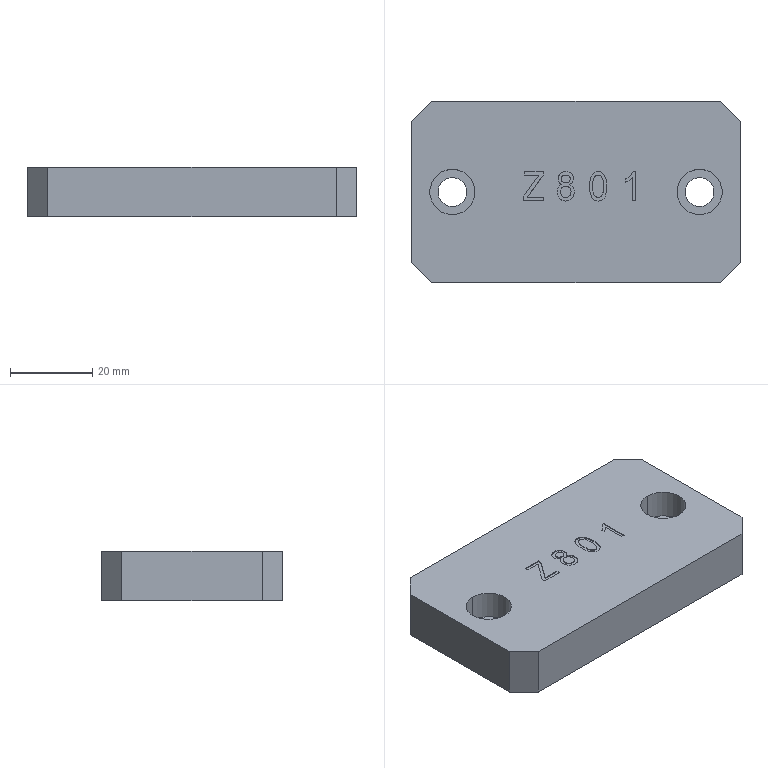Part | Creo | 1 solid | 101 faces | box 80 x 44 x 12 mm | volume 39915 mm3 | other 59 | plane 32 | cylinder 10 | commonest cylinder face diameters 7 x4 11 x4 3.516 x1 96.185 x1